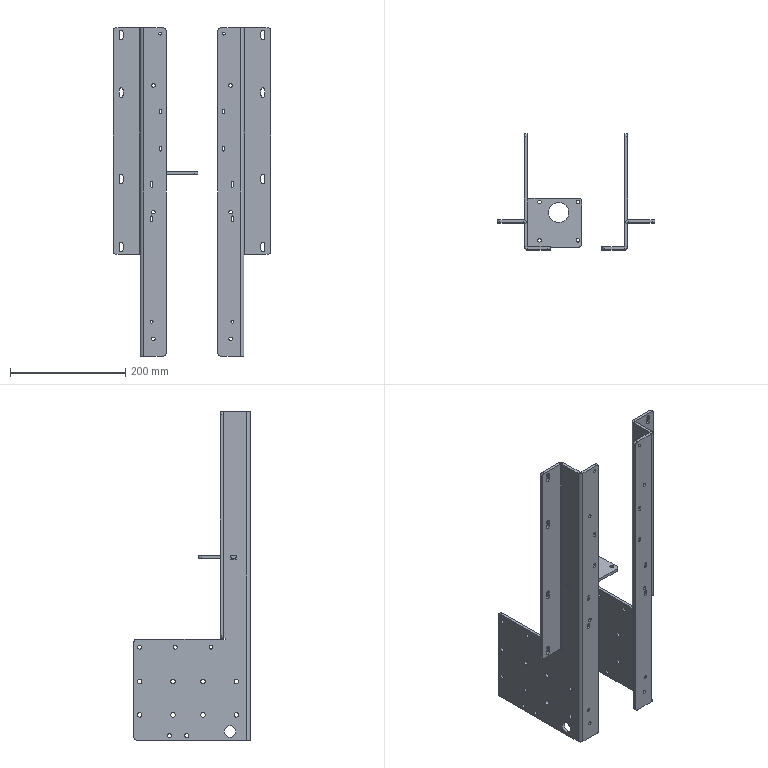Part | SolidWorks | features HoleWzd 9, FlatPattern 3, ICE 3, EdgeFlange 2, Fillet 2, SMBaseFlange 2, SheetMetal 2, TabAndSlotFeature 2, Cut 1, DeleteBody 1, MirrorSolid 1 | 3 solids | 248 faces | box 274 x 202 x 570 mm | volume 975509 mm3 | cylinder 152 | plane 96 | commonest cylinder face diameters 8 x32 4.2 x24 6.8 x20 6.6 x16 10 x16 6 x12